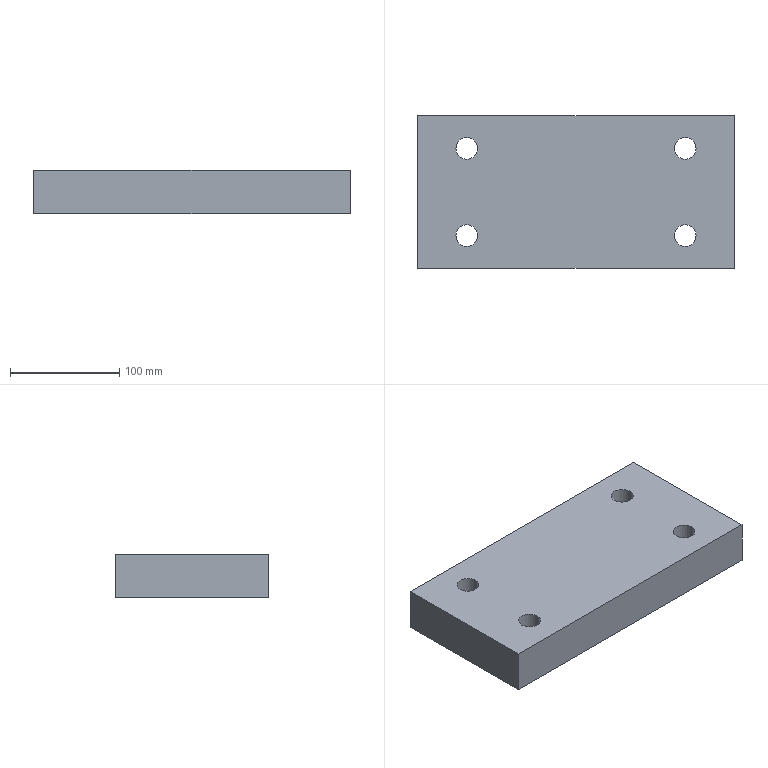Part | SolidWorks | features Extrusion 1 | 1 solid | 14 faces | box 290 x 140 x 40 mm | volume 1573735 mm3 | cylinder 8 | plane 6 | commonest cylinder face diameters 20 x8
STEP:
#1=CARTESIAN_POINT('',(90.,40.,40.));
#2=VERTEX_POINT('',#1);
#3=CARTESIAN_POINT('',(110.,40.,40.));
#4=VERTEX_POINT('',#3);
#5=CARTESIAN_POINT('',(100.,40.,40.));
#6=DIRECTION('',(0.,0.,1.));
#7=DIRECTION('',(-1.,0.,0.));
#8=AXIS2_PLACEMENT_3D('',#5,#6,#7);
#9=CIRCLE('',#8,10.);
#10=EDGE_CURVE('',#2,#4,#9,.T.);
#11=ORIENTED_EDGE('',*,*,#10,.T.);
#12=CARTESIAN_POINT('',(110.,40.,0.));
#13=VERTEX_POINT('',#12);
#14=CARTESIAN_POINT('',(110.,40.,40.));
#15=DIRECTION('',(0.,0.,-1.));
#16=VECTOR('',#15,1000.);
#17=LINE('',#14,#16);
#18=EDGE_CURVE('',#4,#13,#17,.T.);
#19=ORIENTED_EDGE('',*,*,#18,.T.);
#20=CARTESIAN_POINT('',(90.,40.,0.));
#21=VERTEX_POINT('',#20);
#22=CARTESIAN_POINT('',(100.,40.,0.));
#23=DIRECTION('',(0.,0.,1.));
#24=DIRECTION('',(-1.,0.,0.));
#25=AXIS2_PLACEMENT_3D('',#22,#23,#24);
#26=CIRCLE('',#25,10.);
#27=EDGE_CURVE('',#21,#13,#26,.T.);
#28=ORIENTED_EDGE('',*,*,#27,.F.);
#29=CARTESIAN_POINT('',(90.,40.,40.));
#30=DIRECTION('',(0.,0.,-1.));
#31=VECTOR('',#30,1000.);
#32=LINE('',#29,#31);
#33=EDGE_CURVE('',#2,#21,#32,.T.);
#34=ORIENTED_EDGE('',*,*,#33,.F.);
#35=EDGE_LOOP('',(#11,#19,#28,#34));
#36=FACE_OUTER_BOUND('',#35,.T.);
#37=CARTESIAN_POINT('',(100.,40.,40.));
#38=DIRECTION('',(0.,0.,-1.));
#39=DIRECTION('',(-1.,0.,0.));
#40=AXIS2_PLACEMENT_3D('',#37,#38,#39);
#41=CYLINDRICAL_SURFACE('',#40,10.);
#42=ADVANCED_FACE('',(#36),#41,.F.);
#43=CARTESIAN_POINT('',(90.,-40.,40.));
#44=VERTEX_POINT('',#43);
#45=CARTESIAN_POINT('',(110.,-40.,40.));
#46=VERTEX_POINT('',#45);
#47=CARTESIAN_POINT('',(100.,-40.,40.));
#48=DIRECTION('',(0.,0.,1.));
#49=DIRECTION('',(-1.,0.,0.));
#50=AXIS2_PLACEMENT_3D('',#47,#48,#49);
#51=CIRCLE('',#50,10.);
#52=EDGE_CURVE('',#44,#46,#51,.T.);
#53=ORIENTED_EDGE('',*,*,#52,.T.);
#54=CARTESIAN_POINT('',(110.,-40.,0.));
#55=VERTEX_POINT('',#54);
#56=CARTESIAN_POINT('',(110.,-40.,40.));
#57=DIRECTION('',(0.,0.,-1.));
#58=VECTOR('',#57,1000.);
#59=LINE('',#56,#58);
#60=EDGE_CURVE('',#46,#55,#59,.T.);
#61=ORIENTED_EDGE('',*,*,#60,.T.);
#62=CARTESIAN_POINT('',(90.,-40.,0.));
#63=VERTEX_POINT('',#62);
#64=CARTESIAN_POINT('',(100.,-40.,0.));
#65=DIRECTION('',(0.,0.,1.));
#66=DIRECTION('',(-1.,0.,0.));
#67=AXIS2_PLACEMENT_3D('',#64,#65,#66);
#68=CIRCLE('',#67,10.);
#69=EDGE_CURVE('',#63,#55,#68,.T.);
#70=ORIENTED_EDGE('',*,*,#69,.F.);
#71=CARTESIAN_POINT('',(90.,-40.,40.));
#72=DIRECTION('',(0.,0.,-1.));
#73=VECTOR('',#72,1000.);
#74=LINE('',#71,#73);
#75=EDGE_CURVE('',#44,#63,#74,.T.);
#76=ORIENTED_EDGE('',*,*,#75,.F.);
#77=EDGE_LOOP('',(#53,#61,#70,#76));
#78=FACE_OUTER_BOUND('',#77,.T.);
#79=CARTESIAN_POINT('',(100.,-40.,40.));
#80=DIRECTION('',(0.,0.,-1.));
#81=DIRECTION('',(-1.,0.,0.));
#82=AXIS2_PLACEMENT_3D('',#79,#80,#81);
#83=CYLINDRICAL_SURFACE('',#82,10.);
#84=ADVANCED_FACE('',(#78),#83,.F.);
#85=CARTESIAN_POINT('',(-110.,-40.,40.));
#86=VERTEX_POINT('',#85);
#87=CARTESIAN_POINT('',(-90.,-40.,40.));
#88=VERTEX_POINT('',#87);
#89=CARTESIAN_POINT('',(-100.,-40.,40.));
#90=DIRECTION('',(0.,0.,1.));
#91=DIRECTION('',(1.,0.,0.));
#92=AXIS2_PLACEMENT_3D('',#89,#90,#91);
#93=CIRCLE('',#92,10.);
#94=EDGE_CURVE('',#86,#88,#93,.T.);
#95=ORIENTED_EDGE('',*,*,#94,.T.);
#96=CARTESIAN_POINT('',(-90.,-40.,0.));
#97=VERTEX_POINT('',#96);
#98=CARTESIAN_POINT('',(-90.,-40.,40.));
#99=DIRECTION('',(0.,0.,-1.));
#100=VECTOR('',#99,1000.);
#101=LINE('',#98,#100);
#102=EDGE_CURVE('',#88,#97,#101,.T.);
#103=ORIENTED_EDGE('',*,*,#102,.T.);
#104=CARTESIAN_POINT('',(-110.,-40.,0.));
#105=VERTEX_POINT('',#104);
#106=CARTESIAN_POINT('',(-100.,-40.,0.));
#107=DIRECTION('',(0.,0.,1.));
#108=DIRECTION('',(1.,0.,0.));
#109=AXIS2_PLACEMENT_3D('',#106,#107,#108);
#110=CIRCLE('',#109,10.);
#111=EDGE_CURVE('',#105,#97,#110,.T.);
#112=ORIENTED_EDGE('',*,*,#111,.F.);
#113=CARTESIAN_POINT('',(-110.,-40.,40.));
#114=DIRECTION('',(0.,0.,-1.));
#115=VECTOR('',#114,1000.);
#116=LINE('',#113,#115);
#117=EDGE_CURVE('',#86,#105,#116,.T.);
#118=ORIENTED_EDGE('',*,*,#117,.F.);
#119=EDGE_LOOP('',(#95,#103,#112,#118));
#120=FACE_OUTER_BOUND('',#119,.T.);
#121=CARTESIAN_POINT('',(-100.,-40.,40.));
#122=DIRECTION('',(0.,0.,-1.));
#123=DIRECTION('',(-1.,0.,0.));
#124=AXIS2_PLACEMENT_3D('',#121,#122,#123);
#125=CYLINDRICAL_SURFACE('',#124,10.);
#126=ADVANCED_FACE('',(#120),#125,.F.);
#127=CARTESIAN_POINT('',(-110.,40.,40.));
#128=VERTEX_POINT('',#127);
#129=CARTESIAN_POINT('',(-90.,40.,40.));
#130=VERTEX_POINT('',#129);
#131=CARTESIAN_POINT('',(-100.,40.,40.));
#132=DIRECTION('',(0.,0.,1.));
#133=DIRECTION('',(1.,0.,0.));
#134=AXIS2_PLACEMENT_3D('',#131,#132,#133);
#135=CIRCLE('',#134,10.);
#136=EDGE_CURVE('',#128,#130,#135,.T.);
#137=ORIENTED_EDGE('',*,*,#136,.T.);
#138=CARTESIAN_POINT('',(-90.,40.,0.));
#139=VERTEX_POINT('',#138);
#140=CARTESIAN_POINT('',(-90.,40.,40.));
#141=DIRECTION('',(0.,0.,-1.));
#142=VECTOR('',#141,1000.);
#143=LINE('',#140,#142);
#144=EDGE_CURVE('',#130,#139,#143,.T.);
#145=ORIENTED_EDGE('',*,*,#144,.T.);
#146=CARTESIAN_POINT('',(-110.,40.,0.));
#147=VERTEX_POINT('',#146);
#148=CARTESIAN_POINT('',(-100.,40.,0.));
#149=DIRECTION('',(0.,0.,1.));
#150=DIRECTION('',(1.,0.,0.));
#151=AXIS2_PLACEMENT_3D('',#148,#149,#150);
#152=CIRCLE('',#151,10.);
#153=EDGE_CURVE('',#147,#139,#152,.T.);
#154=ORIENTED_EDGE('',*,*,#153,.F.);
#155=CARTESIAN_POINT('',(-110.,40.,40.));
#156=DIRECTION('',(0.,0.,-1.));
#157=VECTOR('',#156,1000.);
#158=LINE('',#155,#157);
#159=EDGE_CURVE('',#128,#147,#158,.T.);
#160=ORIENTED_EDGE('',*,*,#159,.F.);
#161=EDGE_LOOP('',(#137,#145,#154,#160));
#162=FACE_OUTER_BOUND('',#161,.T.);
#163=CARTESIAN_POINT('',(-100.,40.,40.));
#164=DIRECTION('',(0.,0.,-1.));
#165=DIRECTION('',(-1.,0.,0.));
#166=AXIS2_PLACEMENT_3D('',#163,#164,#165);
#167=CYLINDRICAL_SURFACE('',#166,10.);
#168=ADVANCED_FACE('',(#162),#167,.F.);
#169=CARTESIAN_POINT('',(145.,-70.,40.));
#170=VERTEX_POINT('',#169);
#171=CARTESIAN_POINT('',(145.,70.,40.));
#172=VERTEX_POINT('',#171);
#173=CARTESIAN_POINT('',(145.,-70.,40.));
#174=DIRECTION('',(0.,1.,0.));
#175=VECTOR('',#174,1000.);
#176=LINE('',#173,#175);
#177=EDGE_CURVE('',#170,#172,#176,.T.);
#178=ORIENTED_EDGE('',*,*,#177,.T.);
#179=CARTESIAN_POINT('',(-145.,70.,40.));
#180=VERTEX_POINT('',#179);
#181=CARTESIAN_POINT('',(-145.,70.,40.));
#182=DIRECTION('',(-1.,0.,0.));
#183=VECTOR('',#182,1000.);
#184=LINE('',#181,#183);
#185=EDGE_CURVE('',#172,#180,#184,.T.);
#186=ORIENTED_EDGE('',*,*,#185,.T.);
#187=CARTESIAN_POINT('',(-145.,-70.,40.));
#188=VERTEX_POINT('',#187);
#189=CARTESIAN_POINT('',(-145.,-70.,40.));
#190=DIRECTION('',(0.,-1.,0.));
#191=VECTOR('',#190,1000.);
#192=LINE('',#189,#191);
#193=EDGE_CURVE('',#180,#188,#192,.T.);
#194=ORIENTED_EDGE('',*,*,#193,.T.);
#195=CARTESIAN_POINT('',(-145.,-70.,40.));
#196=DIRECTION('',(1.,0.,0.));
#197=VECTOR('',#196,1000.);
#198=LINE('',#195,#197);
#199=EDGE_CURVE('',#188,#170,#198,.T.);
#200=ORIENTED_EDGE('',*,*,#199,.T.);
#201=EDGE_LOOP('',(#178,#186,#194,#200));
#202=FACE_OUTER_BOUND('',#201,.T.);
#203=ORIENTED_EDGE('',*,*,#136,.F.);
#204=CARTESIAN_POINT('',(-100.,40.,40.));
#205=DIRECTION('',(0.,0.,1.));
#206=DIRECTION('',(1.,0.,0.));
#207=AXIS2_PLACEMENT_3D('',#204,#205,#206);
#208=CIRCLE('',#207,10.);
#209=EDGE_CURVE('',#130,#128,#208,.T.);
#210=ORIENTED_EDGE('',*,*,#209,.F.);
#211=EDGE_LOOP('',(#203,#210));
#212=FACE_BOUND('',#211,.T.);
#213=ORIENTED_EDGE('',*,*,#94,.F.);
#214=CARTESIAN_POINT('',(-100.,-40.,40.));
#215=DIRECTION('',(0.,0.,1.));
#216=DIRECTION('',(1.,0.,0.));
#217=AXIS2_PLACEMENT_3D('',#214,#215,#216);
#218=CIRCLE('',#217,10.);
#219=EDGE_CURVE('',#88,#86,#218,.T.);
#220=ORIENTED_EDGE('',*,*,#219,.F.);
#221=EDGE_LOOP('',(#213,#220));
#222=FACE_BOUND('',#221,.T.);
#223=ORIENTED_EDGE('',*,*,#52,.F.);
#224=CARTESIAN_POINT('',(100.,-40.,40.));
#225=DIRECTION('',(0.,0.,1.));
#226=DIRECTION('',(-1.,0.,0.));
#227=AXIS2_PLACEMENT_3D('',#224,#225,#226);
#228=CIRCLE('',#227,10.);
#229=EDGE_CURVE('',#46,#44,#228,.T.);
#230=ORIENTED_EDGE('',*,*,#229,.F.);
#231=EDGE_LOOP('',(#223,#230));
#232=FACE_BOUND('',#231,.T.);
#233=ORIENTED_EDGE('',*,*,#10,.F.);
#234=CARTESIAN_POINT('',(100.,40.,40.));
#235=DIRECTION('',(0.,0.,1.));
#236=DIRECTION('',(-1.,0.,0.));
#237=AXIS2_PLACEMENT_3D('',#234,#235,#236);
#238=CIRCLE('',#237,10.);
#239=EDGE_CURVE('',#4,#2,#238,.T.);
#240=ORIENTED_EDGE('',*,*,#239,.F.);
#241=EDGE_LOOP('',(#233,#240));
#242=FACE_BOUND('',#241,.T.);
#243=CARTESIAN_POINT('',(0.,0.,40.));
#244=DIRECTION('',(0.,0.,-1.));
#245=DIRECTION('',(-1.,0.,0.));
#246=AXIS2_PLACEMENT_3D('',#243,#244,#245);
#247=PLANE('',#246);
#248=ADVANCED_FACE('',(#202,#212,#222,#232,#242),#247,.F.);
#249=ORIENTED_EDGE('',*,*,#69,.T.);
#250=CARTESIAN_POINT('',(100.,-40.,0.));
#251=DIRECTION('',(0.,0.,1.));
#252=DIRECTION('',(-1.,0.,0.));
#253=AXIS2_PLACEMENT_3D('',#250,#251,#252);
#254=CIRCLE('',#253,10.);
#255=EDGE_CURVE('',#55,#63,#254,.T.);
#256=ORIENTED_EDGE('',*,*,#255,.T.);
#257=EDGE_LOOP('',(#249,#256));
#258=FACE_BOUND('',#257,.T.);
#259=ORIENTED_EDGE('',*,*,#153,.T.);
#260=CARTESIAN_POINT('',(-100.,40.,0.));
#261=DIRECTION('',(0.,0.,1.));
#262=DIRECTION('',(1.,0.,0.));
#263=AXIS2_PLACEMENT_3D('',#260,#261,#262);
#264=CIRCLE('',#263,10.);
#265=EDGE_CURVE('',#139,#147,#264,.T.);
#266=ORIENTED_EDGE('',*,*,#265,.T.);
#267=EDGE_LOOP('',(#259,#266));
#268=FACE_BOUND('',#267,.T.);
#269=CARTESIAN_POINT('',(145.,-70.,0.));
#270=VERTEX_POINT('',#269);
#271=CARTESIAN_POINT('',(145.,70.,0.));
#272=VERTEX_POINT('',#271);
#273=CARTESIAN_POINT('',(145.,-70.,0.));
#274=DIRECTION('',(0.,1.,0.));
#275=VECTOR('',#274,1000.);
#276=LINE('',#273,#275);
#277=EDGE_CURVE('',#270,#272,#276,.T.);
#278=ORIENTED_EDGE('',*,*,#277,.F.);
#279=CARTESIAN_POINT('',(-145.,-70.,0.));
#280=VERTEX_POINT('',#279);
#281=CARTESIAN_POINT('',(-145.,-70.,0.));
#282=DIRECTION('',(1.,0.,0.));
#283=VECTOR('',#282,1000.);
#284=LINE('',#281,#283);
#285=EDGE_CURVE('',#280,#270,#284,.T.);
#286=ORIENTED_EDGE('',*,*,#285,.F.);
#287=CARTESIAN_POINT('',(-145.,70.,0.));
#288=VERTEX_POINT('',#287);
#289=CARTESIAN_POINT('',(-145.,-70.,0.));
#290=DIRECTION('',(0.,-1.,0.));
#291=VECTOR('',#290,1000.);
#292=LINE('',#289,#291);
#293=EDGE_CURVE('',#288,#280,#292,.T.);
#294=ORIENTED_EDGE('',*,*,#293,.F.);
#295=CARTESIAN_POINT('',(-145.,70.,0.));
#296=DIRECTION('',(-1.,0.,0.));
#297=VECTOR('',#296,1000.);
#298=LINE('',#295,#297);
#299=EDGE_CURVE('',#272,#288,#298,.T.);
#300=ORIENTED_EDGE('',*,*,#299,.F.);
#301=EDGE_LOOP('',(#278,#286,#294,#300));
#302=FACE_OUTER_BOUND('',#301,.T.);
#303=ORIENTED_EDGE('',*,*,#111,.T.);
#304=CARTESIAN_POINT('',(-100.,-40.,0.));
#305=DIRECTION('',(0.,0.,1.));
#306=DIRECTION('',(1.,0.,0.));
#307=AXIS2_PLACEMENT_3D('',#304,#305,#306);
#308=CIRCLE('',#307,10.);
#309=EDGE_CURVE('',#97,#105,#308,.T.);
#310=ORIENTED_EDGE('',*,*,#309,.T.);
#311=EDGE_LOOP('',(#303,#310));
#312=FACE_BOUND('',#311,.T.);
#313=ORIENTED_EDGE('',*,*,#27,.T.);
#314=CARTESIAN_POINT('',(100.,40.,0.));
#315=DIRECTION('',(0.,0.,1.));
#316=DIRECTION('',(-1.,0.,0.));
#317=AXIS2_PLACEMENT_3D('',#314,#315,#316);
#318=CIRCLE('',#317,10.);
#319=EDGE_CURVE('',#13,#21,#318,.T.);
#320=ORIENTED_EDGE('',*,*,#319,.T.);
#321=EDGE_LOOP('',(#313,#320));
#322=FACE_BOUND('',#321,.T.);
#323=CARTESIAN_POINT('',(0.,0.,0.));
#324=DIRECTION('',(0.,0.,-1.));
#325=DIRECTION('',(-1.,0.,0.));
#326=AXIS2_PLACEMENT_3D('',#323,#324,#325);
#327=PLANE('',#326);
#328=ADVANCED_FACE('',(#258,#268,#302,#312,#322),#327,.T.);
#329=ORIENTED_EDGE('',*,*,#277,.T.);
#330=CARTESIAN_POINT('',(145.,70.,40.));
#331=DIRECTION('',(0.,0.,-1.));
#332=VECTOR('',#331,1000.);
#333=LINE('',#330,#332);
#334=EDGE_CURVE('',#172,#272,#333,.T.);
#335=ORIENTED_EDGE('',*,*,#334,.F.);
#336=ORIENTED_EDGE('',*,*,#177,.F.);
#337=CARTESIAN_POINT('',(145.,-70.,40.));
#338=DIRECTION('',(0.,0.,-1.));
#339=VECTOR('',#338,1000.);
#340=LINE('',#337,#339);
#341=EDGE_CURVE('',#170,#270,#340,.T.);
#342=ORIENTED_EDGE('',*,*,#341,.T.);
#343=EDGE_LOOP('',(#329,#335,#336,#342));
#344=FACE_OUTER_BOUND('',#343,.T.);
#345=CARTESIAN_POINT('',(145.,-70.,40.));
#346=DIRECTION('',(-1.,0.,0.));
#347=DIRECTION('',(0.,0.,1.));
#348=AXIS2_PLACEMENT_3D('',#345,#346,#347);
#349=PLANE('',#348);
#350=ADVANCED_FACE('',(#344),#349,.F.);
#351=ORIENTED_EDGE('',*,*,#299,.T.);
#352=CARTESIAN_POINT('',(-145.,70.,40.));
#353=DIRECTION('',(0.,0.,-1.));
#354=VECTOR('',#353,1000.);
#355=LINE('',#352,#354);
#356=EDGE_CURVE('',#180,#288,#355,.T.);
#357=ORIENTED_EDGE('',*,*,#356,.F.);
#358=ORIENTED_EDGE('',*,*,#185,.F.);
#359=ORIENTED_EDGE('',*,*,#334,.T.);
#360=EDGE_LOOP('',(#351,#357,#358,#359));
#361=FACE_OUTER_BOUND('',#360,.T.);
#362=CARTESIAN_POINT('',(-145.,70.,40.));
#363=DIRECTION('',(0.,-1.,0.));
#364=DIRECTION('',(0.,0.,-1.));
#365=AXIS2_PLACEMENT_3D('',#362,#363,#364);
#366=PLANE('',#365);
#367=ADVANCED_FACE('',(#361),#366,.F.);
#368=ORIENTED_EDGE('',*,*,#293,.T.);
#369=CARTESIAN_POINT('',(-145.,-70.,40.));
#370=DIRECTION('',(0.,0.,-1.));
#371=VECTOR('',#370,1000.);
#372=LINE('',#369,#371);
#373=EDGE_CURVE('',#188,#280,#372,.T.);
#374=ORIENTED_EDGE('',*,*,#373,.F.);
#375=ORIENTED_EDGE('',*,*,#193,.F.);
#376=ORIENTED_EDGE('',*,*,#356,.T.);
#377=EDGE_LOOP('',(#368,#374,#375,#376));
#378=FACE_OUTER_BOUND('',#377,.T.);
#379=CARTESIAN_POINT('',(-145.,-70.,40.));
#380=DIRECTION('',(1.,0.,0.));
#381=DIRECTION('',(0.,0.,-1.));
#382=AXIS2_PLACEMENT_3D('',#379,#380,#381);
#383=PLANE('',#382);
#384=ADVANCED_FACE('',(#378),#383,.F.);
#385=ORIENTED_EDGE('',*,*,#285,.T.);
#386=ORIENTED_EDGE('',*,*,#341,.F.);
#387=ORIENTED_EDGE('',*,*,#199,.F.);
#388=ORIENTED_EDGE('',*,*,#373,.T.);
#389=EDGE_LOOP('',(#385,#386,#387,#388));
#390=FACE_OUTER_BOUND('',#389,.T.);
#391=CARTESIAN_POINT('',(-145.,-70.,40.));
#392=DIRECTION('',(0.,1.,0.));
#393=DIRECTION('',(0.,0.,1.));
#394=AXIS2_PLACEMENT_3D('',#391,#392,#393);
#395=PLANE('',#394);
#396=ADVANCED_FACE('',(#390),#395,.F.);
#397=ORIENTED_EDGE('',*,*,#144,.F.);
#398=ORIENTED_EDGE('',*,*,#209,.T.);
#399=ORIENTED_EDGE('',*,*,#159,.T.);
#400=ORIENTED_EDGE('',*,*,#265,.F.);
#401=EDGE_LOOP('',(#397,#398,#399,#400));
#402=FACE_OUTER_BOUND('',#401,.T.);
#403=CARTESIAN_POINT('',(-100.,40.,40.));
#404=DIRECTION('',(0.,0.,-1.));
#405=DIRECTION('',(-1.,0.,0.));
#406=AXIS2_PLACEMENT_3D('',#403,#404,#405);
#407=CYLINDRICAL_SURFACE('',#406,10.);
#408=ADVANCED_FACE('',(#402),#407,.F.);
#409=ORIENTED_EDGE('',*,*,#102,.F.);
#410=ORIENTED_EDGE('',*,*,#219,.T.);
#411=ORIENTED_EDGE('',*,*,#117,.T.);
#412=ORIENTED_EDGE('',*,*,#309,.F.);
#413=EDGE_LOOP('',(#409,#410,#411,#412));
#414=FACE_OUTER_BOUND('',#413,.T.);
#415=CARTESIAN_POINT('',(-100.,-40.,40.));
#416=DIRECTION('',(0.,0.,-1.));
#417=DIRECTION('',(-1.,0.,0.));
#418=AXIS2_PLACEMENT_3D('',#415,#416,#417);
#419=CYLINDRICAL_SURFACE('',#418,10.);
#420=ADVANCED_FACE('',(#414),#419,.F.);
#421=ORIENTED_EDGE('',*,*,#60,.F.);
#422=ORIENTED_EDGE('',*,*,#229,.T.);
#423=ORIENTED_EDGE('',*,*,#75,.T.);
#424=ORIENTED_EDGE('',*,*,#255,.F.);
#425=EDGE_LOOP('',(#421,#422,#423,#424));
#426=FACE_OUTER_BOUND('',#425,.T.);
#427=CARTESIAN_POINT('',(100.,-40.,40.));
#428=DIRECTION('',(0.,0.,-1.));
#429=DIRECTION('',(-1.,0.,0.));
#430=AXIS2_PLACEMENT_3D('',#427,#428,#429);
#431=CYLINDRICAL_SURFACE('',#430,10.);
#432=ADVANCED_FACE('',(#426),#431,.F.);
#433=ORIENTED_EDGE('',*,*,#18,.F.);
#434=ORIENTED_EDGE('',*,*,#239,.T.);
#435=ORIENTED_EDGE('',*,*,#33,.T.);
#436=ORIENTED_EDGE('',*,*,#319,.F.);
#437=EDGE_LOOP('',(#433,#434,#435,#436));
#438=FACE_OUTER_BOUND('',#437,.T.);
#439=CARTESIAN_POINT('',(100.,40.,40.));
#440=DIRECTION('',(0.,0.,-1.));
#441=DIRECTION('',(-1.,0.,0.));
#442=AXIS2_PLACEMENT_3D('',#439,#440,#441);
#443=CYLINDRICAL_SURFACE('',#442,10.);
#444=ADVANCED_FACE('',(#438),#443,.F.);
#445=CLOSED_SHELL('',(#42,#84,#126,#168,#248,#328,#350,#367,#384,#396,#408,#420,#432,#444));
#446=MANIFOLD_SOLID_BREP('',#445);
#447=CARTESIAN_POINT('',(0.,0.,0.));
#448=DIRECTION('',(0.,0.,1.));
#449=DIRECTION('',(1.,0.,0.));
#450=AXIS2_PLACEMENT_3D('',#447,#448,#449);
#451=(LENGTH_UNIT()NAMED_UNIT(*)SI_UNIT(.MILLI.,.METRE.));
#452=UNCERTAINTY_MEASURE_WITH_UNIT(LENGTH_MEASURE(0.00001),#451,'','');
#453=(NAMED_UNIT(*)PLANE_ANGLE_UNIT()SI_UNIT($,.RADIAN.));
#454=(NAMED_UNIT(*)SI_UNIT($,.STERADIAN.)SOLID_ANGLE_UNIT());
#455=(GEOMETRIC_REPRESENTATION_CONTEXT(3)GLOBAL_UNCERTAINTY_ASSIGNED_CONTEXT((#452))GLOBAL_UNIT_ASSIGNED_CONTEXT((#451,#453,#454))REPRESENTATION_CONTEXT('',''));
#456=ADVANCED_BREP_SHAPE_REPRESENTATION('',(#446,#450),#455);